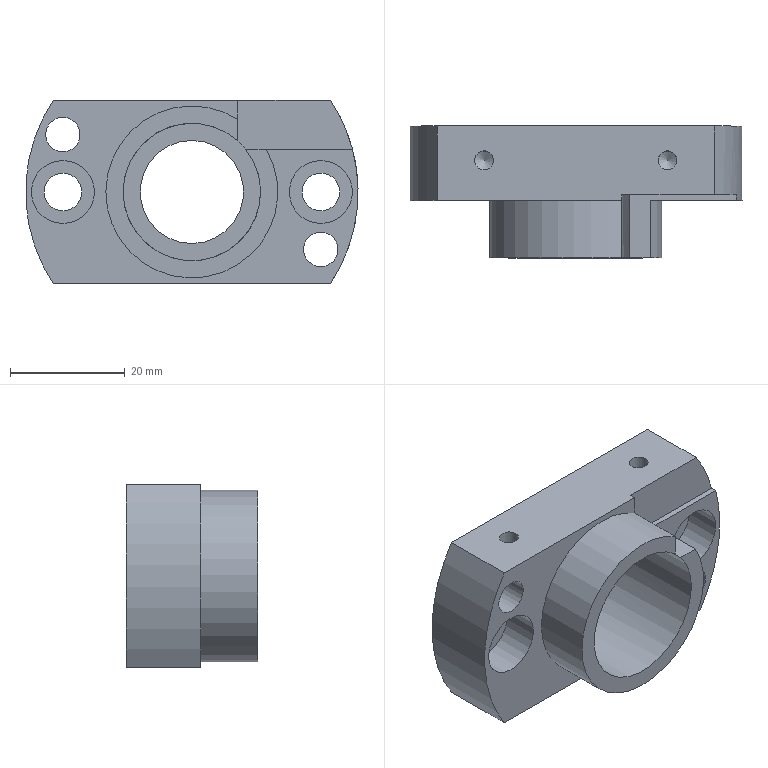Part | NX | features BREP 1 | 1 solid | 26 faces | box 58 x 23 x 32 mm | volume 17221 mm3 | cylinder 13 | plane 11 | cone 2 | commonest cylinder face diameters 3.3 x2 6 x2 6.6 x2 11 x2 58 x2 18 x1
STEP:
#1=CARTESIAN_POINT('',(9.367,11.,7.5));
#2=VERTEX_POINT('',#1);
#3=CARTESIAN_POINT('',(8.,11.,8.944));
#4=VERTEX_POINT('',#3);
#5=CARTESIAN_POINT('',(0.,11.,0.));
#6=DIRECTION('',(0.,-1.,0.));
#7=DIRECTION('',(0.,0.,1.));
#8=AXIS2_PLACEMENT_3D('',#5,#6,#7);
#9=CIRCLE('',#8,12.);
#10=EDGE_CURVE('',#2,#4,#9,.T.);
#11=ORIENTED_EDGE('',*,*,#10,.T.);
#12=CARTESIAN_POINT('',(8.,0.,8.944));
#13=VERTEX_POINT('',#12);
#14=CARTESIAN_POINT('',(8.,0.,8.944));
#15=DIRECTION('',(0.,-1.,0.));
#16=VECTOR('',#15,1000.);
#17=LINE('',#14,#16);
#18=EDGE_CURVE('',#4,#13,#17,.T.);
#19=ORIENTED_EDGE('',*,*,#18,.T.);
#20=CARTESIAN_POINT('',(9.367,0.,7.5));
#21=VERTEX_POINT('',#20);
#22=CARTESIAN_POINT('',(0.,0.,0.));
#23=DIRECTION('',(0.,1.,0.));
#24=DIRECTION('',(0.,0.,1.));
#25=AXIS2_PLACEMENT_3D('',#22,#23,#24);
#26=CIRCLE('',#25,12.);
#27=EDGE_CURVE('',#21,#13,#26,.T.);
#28=ORIENTED_EDGE('',*,*,#27,.F.);
#29=CARTESIAN_POINT('',(9.367,0.,7.5));
#30=DIRECTION('',(0.,1.,0.));
#31=VECTOR('',#30,1000.);
#32=LINE('',#29,#31);
#33=EDGE_CURVE('',#21,#2,#32,.T.);
#34=ORIENTED_EDGE('',*,*,#33,.T.);
#35=EDGE_LOOP('',(#11,#19,#28,#34));
#36=FACE_BOUND('',#35,.T.);
#37=CARTESIAN_POINT('',(0.,20.,12.));
#38=VERTEX_POINT('',#37);
#39=CARTESIAN_POINT('',(0.,20.,0.));
#40=DIRECTION('',(0.,-1.,0.));
#41=DIRECTION('',(0.,0.,1.));
#42=AXIS2_PLACEMENT_3D('',#39,#40,#41);
#43=CIRCLE('',#42,12.);
#44=EDGE_CURVE('',#38,#38,#43,.T.);
#45=ORIENTED_EDGE('',*,*,#44,.F.);
#46=EDGE_LOOP('',(#45));
#47=FACE_BOUND('',#46,.T.);
#48=CARTESIAN_POINT('',(0.,0.,0.));
#49=DIRECTION('',(0.,1.,0.));
#50=DIRECTION('',(0.,0.,-1.));
#51=AXIS2_PLACEMENT_3D('',#48,#49,#50);
#52=CYLINDRICAL_SURFACE('',#51,12.);
#53=ADVANCED_FACE('',(#36,#47),#52,.F.);
#54=CARTESIAN_POINT('',(-22.5,10.,13.));
#55=VERTEX_POINT('',#54);
#56=CARTESIAN_POINT('',(-22.5,10.,10.));
#57=DIRECTION('',(0.,1.,0.));
#58=DIRECTION('',(0.,0.,1.));
#59=AXIS2_PLACEMENT_3D('',#56,#57,#58);
#60=CIRCLE('',#59,3.);
#61=EDGE_CURVE('',#55,#55,#60,.T.);
#62=ORIENTED_EDGE('',*,*,#61,.T.);
#63=EDGE_LOOP('',(#62));
#64=FACE_BOUND('',#63,.T.);
#65=CARTESIAN_POINT('',(22.5,10.,-7.));
#66=VERTEX_POINT('',#65);
#67=CARTESIAN_POINT('',(22.5,10.,-10.));
#68=DIRECTION('',(0.,1.,0.));
#69=DIRECTION('',(0.,0.,1.));
#70=AXIS2_PLACEMENT_3D('',#67,#68,#69);
#71=CIRCLE('',#70,3.);
#72=EDGE_CURVE('',#66,#66,#71,.T.);
#73=ORIENTED_EDGE('',*,*,#72,.T.);
#74=EDGE_LOOP('',(#73));
#75=FACE_BOUND('',#74,.T.);
#76=CARTESIAN_POINT('',(22.5,10.,-5.5));
#77=VERTEX_POINT('',#76);
#78=CARTESIAN_POINT('',(22.5,10.,0.));
#79=DIRECTION('',(0.,-1.,0.));
#80=DIRECTION('',(0.,0.,-1.));
#81=AXIS2_PLACEMENT_3D('',#78,#79,#80);
#82=CIRCLE('',#81,5.5);
#83=EDGE_CURVE('',#77,#77,#82,.T.);
#84=ORIENTED_EDGE('',*,*,#83,.F.);
#85=EDGE_LOOP('',(#84));
#86=FACE_BOUND('',#85,.T.);
#87=CARTESIAN_POINT('',(-22.5,10.,-5.5));
#88=VERTEX_POINT('',#87);
#89=CARTESIAN_POINT('',(-22.5,10.,0.));
#90=DIRECTION('',(0.,-1.,0.));
#91=DIRECTION('',(0.,0.,-1.));
#92=AXIS2_PLACEMENT_3D('',#89,#90,#91);
#93=CIRCLE('',#92,5.5);
#94=EDGE_CURVE('',#88,#88,#93,.T.);
#95=ORIENTED_EDGE('',*,*,#94,.F.);
#96=EDGE_LOOP('',(#95));
#97=FACE_BOUND('',#96,.T.);
#98=CARTESIAN_POINT('',(12.99,10.,7.5));
#99=VERTEX_POINT('',#98);
#100=CARTESIAN_POINT('',(8.,10.,12.689));
#101=VERTEX_POINT('',#100);
#102=CARTESIAN_POINT('',(0.,10.,0.));
#103=DIRECTION('',(0.,1.,0.));
#104=DIRECTION('',(0.,0.,1.));
#105=AXIS2_PLACEMENT_3D('',#102,#103,#104);
#106=CIRCLE('',#105,15.);
#107=EDGE_CURVE('',#99,#101,#106,.T.);
#108=ORIENTED_EDGE('',*,*,#107,.T.);
#109=CARTESIAN_POINT('',(8.,10.,16.));
#110=VERTEX_POINT('',#109);
#111=CARTESIAN_POINT('',(8.,10.,0.));
#112=DIRECTION('',(0.,0.,1.));
#113=VECTOR('',#112,1000.);
#114=LINE('',#111,#113);
#115=EDGE_CURVE('',#101,#110,#114,.T.);
#116=ORIENTED_EDGE('',*,*,#115,.T.);
#117=CARTESIAN_POINT('',(-24.187,10.,16.));
#118=VERTEX_POINT('',#117);
#119=CARTESIAN_POINT('',(-24.187,10.,16.));
#120=DIRECTION('',(1.,0.,0.));
#121=VECTOR('',#120,1000.);
#122=LINE('',#119,#121);
#123=EDGE_CURVE('',#118,#110,#122,.T.);
#124=ORIENTED_EDGE('',*,*,#123,.F.);
#125=CARTESIAN_POINT('',(-24.187,10.,-16.));
#126=VERTEX_POINT('',#125);
#127=CARTESIAN_POINT('',(0.,10.,0.));
#128=DIRECTION('',(0.,1.,0.));
#129=DIRECTION('',(0.,0.,1.));
#130=AXIS2_PLACEMENT_3D('',#127,#128,#129);
#131=CIRCLE('',#130,29.);
#132=EDGE_CURVE('',#126,#118,#131,.T.);
#133=ORIENTED_EDGE('',*,*,#132,.F.);
#134=CARTESIAN_POINT('',(24.187,10.,-16.));
#135=VERTEX_POINT('',#134);
#136=CARTESIAN_POINT('',(-24.187,10.,-16.));
#137=DIRECTION('',(1.,0.,0.));
#138=VECTOR('',#137,1000.);
#139=LINE('',#136,#138);
#140=EDGE_CURVE('',#126,#135,#139,.T.);
#141=ORIENTED_EDGE('',*,*,#140,.T.);
#142=CARTESIAN_POINT('',(28.013,10.,7.5));
#143=VERTEX_POINT('',#142);
#144=CARTESIAN_POINT('',(0.,10.,0.));
#145=DIRECTION('',(0.,1.,0.));
#146=DIRECTION('',(0.,0.,1.));
#147=AXIS2_PLACEMENT_3D('',#144,#145,#146);
#148=CIRCLE('',#147,29.);
#149=EDGE_CURVE('',#143,#135,#148,.T.);
#150=ORIENTED_EDGE('',*,*,#149,.F.);
#151=CARTESIAN_POINT('',(15.,10.,7.5));
#152=DIRECTION('',(-1.,0.,0.));
#153=VECTOR('',#152,1000.);
#154=LINE('',#151,#153);
#155=EDGE_CURVE('',#143,#99,#154,.T.);
#156=ORIENTED_EDGE('',*,*,#155,.T.);
#157=EDGE_LOOP('',(#108,#116,#124,#133,#141,#150,#156));
#158=FACE_BOUND('',#157,.T.);
#159=CARTESIAN_POINT('',(15.,10.,0.));
#160=DIRECTION('',(0.,1.,0.));
#161=DIRECTION('',(0.,0.,-1.));
#162=AXIS2_PLACEMENT_3D('',#159,#160,#161);
#163=PLANE('',#162);
#164=ADVANCED_FACE('',(#64,#75,#86,#97,#158),#163,.F.);
#165=CARTESIAN_POINT('',(24.187,11.,16.));
#166=VERTEX_POINT('',#165);
#167=CARTESIAN_POINT('',(28.013,11.,7.5));
#168=VERTEX_POINT('',#167);
#169=CARTESIAN_POINT('',(0.,11.,0.));
#170=DIRECTION('',(0.,1.,0.));
#171=DIRECTION('',(0.,0.,1.));
#172=AXIS2_PLACEMENT_3D('',#169,#170,#171);
#173=CIRCLE('',#172,29.);
#174=EDGE_CURVE('',#166,#168,#173,.T.);
#175=ORIENTED_EDGE('',*,*,#174,.T.);
#176=CARTESIAN_POINT('',(28.013,0.,7.5));
#177=DIRECTION('',(0.,-1.,0.));
#178=VECTOR('',#177,1000.);
#179=LINE('',#176,#178);
#180=EDGE_CURVE('',#168,#143,#179,.T.);
#181=ORIENTED_EDGE('',*,*,#180,.T.);
#182=ORIENTED_EDGE('',*,*,#149,.T.);
#183=CARTESIAN_POINT('',(24.187,23.,-16.));
#184=VERTEX_POINT('',#183);
#185=CARTESIAN_POINT('',(24.187,73.737,-16.));
#186=DIRECTION('',(0.,-1.,0.));
#187=VECTOR('',#186,1000.);
#188=LINE('',#185,#187);
#189=EDGE_CURVE('',#184,#135,#188,.T.);
#190=ORIENTED_EDGE('',*,*,#189,.F.);
#191=CARTESIAN_POINT('',(24.187,23.,16.));
#192=VERTEX_POINT('',#191);
#193=CARTESIAN_POINT('',(0.,23.,0.));
#194=DIRECTION('',(0.,1.,0.));
#195=DIRECTION('',(0.,0.,1.));
#196=AXIS2_PLACEMENT_3D('',#193,#194,#195);
#197=CIRCLE('',#196,29.);
#198=EDGE_CURVE('',#192,#184,#197,.T.);
#199=ORIENTED_EDGE('',*,*,#198,.F.);
#200=CARTESIAN_POINT('',(24.187,73.737,16.));
#201=DIRECTION('',(0.,-1.,0.));
#202=VECTOR('',#201,1000.);
#203=LINE('',#200,#202);
#204=EDGE_CURVE('',#192,#166,#203,.T.);
#205=ORIENTED_EDGE('',*,*,#204,.T.);
#206=EDGE_LOOP('',(#175,#181,#182,#190,#199,#205));
#207=FACE_BOUND('',#206,.T.);
#208=CARTESIAN_POINT('',(0.,0.,0.));
#209=DIRECTION('',(0.,1.,0.));
#210=DIRECTION('',(0.,0.,-1.));
#211=AXIS2_PLACEMENT_3D('',#208,#209,#210);
#212=CYLINDRICAL_SURFACE('',#211,29.);
#213=ADVANCED_FACE('',(#207),#212,.T.);
#214=CARTESIAN_POINT('',(-24.187,23.,-16.));
#215=VERTEX_POINT('',#214);
#216=CARTESIAN_POINT('',(-24.187,73.737,-16.));
#217=DIRECTION('',(0.,-1.,0.));
#218=VECTOR('',#217,1000.);
#219=LINE('',#216,#218);
#220=EDGE_CURVE('',#215,#126,#219,.T.);
#221=ORIENTED_EDGE('',*,*,#220,.T.);
#222=ORIENTED_EDGE('',*,*,#132,.T.);
#223=CARTESIAN_POINT('',(-24.187,23.,16.));
#224=VERTEX_POINT('',#223);
#225=CARTESIAN_POINT('',(-24.187,73.737,16.));
#226=DIRECTION('',(0.,-1.,0.));
#227=VECTOR('',#226,1000.);
#228=LINE('',#225,#227);
#229=EDGE_CURVE('',#224,#118,#228,.T.);
#230=ORIENTED_EDGE('',*,*,#229,.F.);
#231=CARTESIAN_POINT('',(0.,23.,0.));
#232=DIRECTION('',(0.,1.,0.));
#233=DIRECTION('',(0.,0.,1.));
#234=AXIS2_PLACEMENT_3D('',#231,#232,#233);
#235=CIRCLE('',#234,29.);
#236=EDGE_CURVE('',#215,#224,#235,.T.);
#237=ORIENTED_EDGE('',*,*,#236,.F.);
#238=EDGE_LOOP('',(#221,#222,#230,#237));
#239=FACE_BOUND('',#238,.T.);
#240=CARTESIAN_POINT('',(0.,0.,0.));
#241=DIRECTION('',(0.,1.,0.));
#242=DIRECTION('',(0.,0.,-1.));
#243=AXIS2_PLACEMENT_3D('',#240,#241,#242);
#244=CYLINDRICAL_SURFACE('',#243,29.);
#245=ADVANCED_FACE('',(#239),#244,.T.);
#246=CARTESIAN_POINT('',(-22.5,23.,13.));
#247=VERTEX_POINT('',#246);
#248=CARTESIAN_POINT('',(-22.5,23.,10.));
#249=DIRECTION('',(0.,1.,0.));
#250=DIRECTION('',(0.,0.,1.));
#251=AXIS2_PLACEMENT_3D('',#248,#249,#250);
#252=CIRCLE('',#251,3.);
#253=EDGE_CURVE('',#247,#247,#252,.T.);
#254=ORIENTED_EDGE('',*,*,#253,.F.);
#255=EDGE_LOOP('',(#254));
#256=FACE_BOUND('',#255,.T.);
#257=CARTESIAN_POINT('',(22.5,23.,-7.));
#258=VERTEX_POINT('',#257);
#259=CARTESIAN_POINT('',(22.5,23.,-10.));
#260=DIRECTION('',(0.,1.,0.));
#261=DIRECTION('',(0.,0.,1.));
#262=AXIS2_PLACEMENT_3D('',#259,#260,#261);
#263=CIRCLE('',#262,3.);
#264=EDGE_CURVE('',#258,#258,#263,.T.);
#265=ORIENTED_EDGE('',*,*,#264,.F.);
#266=EDGE_LOOP('',(#265));
#267=FACE_BOUND('',#266,.T.);
#268=CARTESIAN_POINT('',(22.5,23.,-3.3));
#269=VERTEX_POINT('',#268);
#270=CARTESIAN_POINT('',(22.5,23.,0.));
#271=DIRECTION('',(0.,-1.,0.));
#272=DIRECTION('',(0.,0.,-1.));
#273=AXIS2_PLACEMENT_3D('',#270,#271,#272);
#274=CIRCLE('',#273,3.3);
#275=EDGE_CURVE('',#269,#269,#274,.T.);
#276=ORIENTED_EDGE('',*,*,#275,.T.);
#277=EDGE_LOOP('',(#276));
#278=FACE_BOUND('',#277,.T.);
#279=CARTESIAN_POINT('',(-22.5,23.,-3.3));
#280=VERTEX_POINT('',#279);
#281=CARTESIAN_POINT('',(-22.5,23.,0.));
#282=DIRECTION('',(0.,-1.,0.));
#283=DIRECTION('',(0.,0.,-1.));
#284=AXIS2_PLACEMENT_3D('',#281,#282,#283);
#285=CIRCLE('',#284,3.3);
#286=EDGE_CURVE('',#280,#280,#285,.T.);
#287=ORIENTED_EDGE('',*,*,#286,.T.);
#288=EDGE_LOOP('',(#287));
#289=FACE_BOUND('',#288,.T.);
#290=CARTESIAN_POINT('',(-24.187,23.,-16.));
#291=DIRECTION('',(-1.,0.,0.));
#292=VECTOR('',#291,1000.);
#293=LINE('',#290,#292);
#294=EDGE_CURVE('',#184,#215,#293,.T.);
#295=ORIENTED_EDGE('',*,*,#294,.T.);
#296=ORIENTED_EDGE('',*,*,#236,.T.);
#297=CARTESIAN_POINT('',(-24.187,23.,16.));
#298=DIRECTION('',(-1.,0.,0.));
#299=VECTOR('',#298,1000.);
#300=LINE('',#297,#299);
#301=EDGE_CURVE('',#192,#224,#300,.T.);
#302=ORIENTED_EDGE('',*,*,#301,.F.);
#303=ORIENTED_EDGE('',*,*,#198,.T.);
#304=EDGE_LOOP('',(#295,#296,#302,#303));
#305=FACE_BOUND('',#304,.T.);
#306=CARTESIAN_POINT('',(0.,23.,9.));
#307=VERTEX_POINT('',#306);
#308=CARTESIAN_POINT('',(0.,23.,0.));
#309=DIRECTION('',(0.,1.,0.));
#310=DIRECTION('',(0.,0.,1.));
#311=AXIS2_PLACEMENT_3D('',#308,#309,#310);
#312=CIRCLE('',#311,9.);
#313=EDGE_CURVE('',#307,#307,#312,.T.);
#314=ORIENTED_EDGE('',*,*,#313,.F.);
#315=EDGE_LOOP('',(#314));
#316=FACE_BOUND('',#315,.T.);
#317=CARTESIAN_POINT('',(29.,23.,0.));
#318=DIRECTION('',(0.,-1.,0.));
#319=DIRECTION('',(0.,0.,1.));
#320=AXIS2_PLACEMENT_3D('',#317,#318,#319);
#321=PLANE('',#320);
#322=ADVANCED_FACE('',(#256,#267,#278,#289,#305,#316),#321,.F.);
#323=ORIENTED_EDGE('',*,*,#27,.T.);
#324=CARTESIAN_POINT('',(8.,0.,12.689));
#325=VERTEX_POINT('',#324);
#326=CARTESIAN_POINT('',(8.,0.,7.5));
#327=DIRECTION('',(0.,0.,-1.));
#328=VECTOR('',#327,1000.);
#329=LINE('',#326,#328);
#330=EDGE_CURVE('',#325,#13,#329,.T.);
#331=ORIENTED_EDGE('',*,*,#330,.F.);
#332=CARTESIAN_POINT('',(12.99,0.,7.5));
#333=VERTEX_POINT('',#332);
#334=CARTESIAN_POINT('',(0.,0.,0.));
#335=DIRECTION('',(0.,1.,0.));
#336=DIRECTION('',(0.,0.,1.));
#337=AXIS2_PLACEMENT_3D('',#334,#335,#336);
#338=CIRCLE('',#337,15.);
#339=EDGE_CURVE('',#333,#325,#338,.T.);
#340=ORIENTED_EDGE('',*,*,#339,.F.);
#341=CARTESIAN_POINT('',(8.,0.,7.5));
#342=DIRECTION('',(1.,0.,0.));
#343=VECTOR('',#342,1000.);
#344=LINE('',#341,#343);
#345=EDGE_CURVE('',#21,#333,#344,.T.);
#346=ORIENTED_EDGE('',*,*,#345,.F.);
#347=EDGE_LOOP('',(#323,#331,#340,#346));
#348=FACE_BOUND('',#347,.T.);
#349=CARTESIAN_POINT('',(12.,0.,0.));
#350=DIRECTION('',(0.,1.,0.));
#351=DIRECTION('',(0.,0.,-1.));
#352=AXIS2_PLACEMENT_3D('',#349,#350,#351);
#353=PLANE('',#352);
#354=ADVANCED_FACE('',(#348),#353,.F.);
#355=ORIENTED_EDGE('',*,*,#339,.T.);
#356=CARTESIAN_POINT('',(8.,0.,12.689));
#357=DIRECTION('',(0.,1.,0.));
#358=VECTOR('',#357,1000.);
#359=LINE('',#356,#358);
#360=EDGE_CURVE('',#325,#101,#359,.T.);
#361=ORIENTED_EDGE('',*,*,#360,.T.);
#362=ORIENTED_EDGE('',*,*,#107,.F.);
#363=CARTESIAN_POINT('',(12.99,0.,7.5));
#364=DIRECTION('',(0.,-1.,0.));
#365=VECTOR('',#364,1000.);
#366=LINE('',#363,#365);
#367=EDGE_CURVE('',#99,#333,#366,.T.);
#368=ORIENTED_EDGE('',*,*,#367,.T.);
#369=EDGE_LOOP('',(#355,#361,#362,#368));
#370=FACE_BOUND('',#369,.T.);
#371=CARTESIAN_POINT('',(0.,0.,0.));
#372=DIRECTION('',(0.,1.,0.));
#373=DIRECTION('',(0.,0.,-1.));
#374=AXIS2_PLACEMENT_3D('',#371,#372,#373);
#375=CYLINDRICAL_SURFACE('',#374,15.);
#376=ADVANCED_FACE('',(#370),#375,.T.);
#377=CARTESIAN_POINT('',(-14.35,17.,16.));
#378=VERTEX_POINT('',#377);
#379=CARTESIAN_POINT('',(-16.,17.,16.));
#380=DIRECTION('',(0.,0.,1.));
#381=DIRECTION('',(1.,0.,0.));
#382=AXIS2_PLACEMENT_3D('',#379,#380,#381);
#383=CIRCLE('',#382,1.65);
#384=EDGE_CURVE('',#378,#378,#383,.T.);
#385=ORIENTED_EDGE('',*,*,#384,.F.);
#386=EDGE_LOOP('',(#385));
#387=FACE_BOUND('',#386,.T.);
#388=CARTESIAN_POINT('',(17.65,17.,16.));
#389=VERTEX_POINT('',#388);
#390=CARTESIAN_POINT('',(16.,17.,16.));
#391=DIRECTION('',(0.,0.,1.));
#392=DIRECTION('',(1.,0.,0.));
#393=AXIS2_PLACEMENT_3D('',#390,#391,#392);
#394=CIRCLE('',#393,1.65);
#395=EDGE_CURVE('',#389,#389,#394,.T.);
#396=ORIENTED_EDGE('',*,*,#395,.F.);
#397=EDGE_LOOP('',(#396));
#398=FACE_BOUND('',#397,.T.);
#399=ORIENTED_EDGE('',*,*,#123,.T.);
#400=CARTESIAN_POINT('',(8.,11.,16.));
#401=VERTEX_POINT('',#400);
#402=CARTESIAN_POINT('',(8.,11.,16.));
#403=DIRECTION('',(0.,-1.,0.));
#404=VECTOR('',#403,1000.);
#405=LINE('',#402,#404);
#406=EDGE_CURVE('',#401,#110,#405,.T.);
#407=ORIENTED_EDGE('',*,*,#406,.F.);
#408=CARTESIAN_POINT('',(-24.187,11.,16.));
#409=DIRECTION('',(1.,0.,0.));
#410=VECTOR('',#409,1000.);
#411=LINE('',#408,#410);
#412=EDGE_CURVE('',#401,#166,#411,.T.);
#413=ORIENTED_EDGE('',*,*,#412,.T.);
#414=ORIENTED_EDGE('',*,*,#204,.F.);
#415=ORIENTED_EDGE('',*,*,#301,.T.);
#416=ORIENTED_EDGE('',*,*,#229,.T.);
#417=EDGE_LOOP('',(#399,#407,#413,#414,#415,#416));
#418=FACE_BOUND('',#417,.T.);
#419=CARTESIAN_POINT('',(-24.187,73.737,16.));
#420=DIRECTION('',(0.,0.,-1.));
#421=DIRECTION('',(1.,0.,0.));
#422=AXIS2_PLACEMENT_3D('',#419,#420,#421);
#423=PLANE('',#422);
#424=ADVANCED_FACE('',(#387,#398,#418),#423,.F.);
#425=ORIENTED_EDGE('',*,*,#189,.T.);
#426=ORIENTED_EDGE('',*,*,#140,.F.);
#427=ORIENTED_EDGE('',*,*,#220,.F.);
#428=ORIENTED_EDGE('',*,*,#294,.F.);
#429=EDGE_LOOP('',(#425,#426,#427,#428));
#430=FACE_BOUND('',#429,.T.);
#431=CARTESIAN_POINT('',(-24.187,73.737,-16.));
#432=DIRECTION('',(0.,0.,-1.));
#433=DIRECTION('',(1.,0.,0.));
#434=AXIS2_PLACEMENT_3D('',#431,#432,#433);
#435=PLANE('',#434);
#436=ADVANCED_FACE('',(#430),#435,.T.);
#437=ORIENTED_EDGE('',*,*,#286,.F.);
#438=EDGE_LOOP('',(#437));
#439=FACE_BOUND('',#438,.T.);
#440=CARTESIAN_POINT('',(-22.5,16.4,-3.3));
#441=VERTEX_POINT('',#440);
#442=CARTESIAN_POINT('',(-22.5,16.4,0.));
#443=DIRECTION('',(0.,-1.,0.));
#444=DIRECTION('',(0.,0.,-1.));
#445=AXIS2_PLACEMENT_3D('',#442,#443,#444);
#446=CIRCLE('',#445,3.3);
#447=EDGE_CURVE('',#441,#441,#446,.T.);
#448=ORIENTED_EDGE('',*,*,#447,.T.);
#449=EDGE_LOOP('',(#448));
#450=FACE_BOUND('',#449,.T.);
#451=CARTESIAN_POINT('',(-22.5,10.,0.));
#452=DIRECTION('',(0.,-1.,0.));
#453=DIRECTION('',(0.,0.,1.));
#454=AXIS2_PLACEMENT_3D('',#451,#452,#453);
#455=CYLINDRICAL_SURFACE('',#454,3.3);
#456=ADVANCED_FACE('',(#439,#450),#455,.F.);
#457=ORIENTED_EDGE('',*,*,#447,.F.);
#458=EDGE_LOOP('',(#457));
#459=FACE_BOUND('',#458,.T.);
#460=CARTESIAN_POINT('',(-22.5,16.4,-5.5));
#461=VERTEX_POINT('',#460);
#462=CARTESIAN_POINT('',(-22.5,16.4,0.));
#463=DIRECTION('',(0.,-1.,0.));
#464=DIRECTION('',(0.,0.,-1.));
#465=AXIS2_PLACEMENT_3D('',#462,#463,#464);
#466=CIRCLE('',#465,5.5);
#467=EDGE_CURVE('',#461,#461,#466,.T.);
#468=ORIENTED_EDGE('',*,*,#467,.T.);
#469=EDGE_LOOP('',(#468));
#470=FACE_BOUND('',#469,.T.);
#471=CARTESIAN_POINT('',(-19.2,16.4,0.));
#472=DIRECTION('',(0.,1.,0.));
#473=DIRECTION('',(0.,0.,-1.));
#474=AXIS2_PLACEMENT_3D('',#471,#472,#473);
#475=PLANE('',#474);
#476=ADVANCED_FACE('',(#459,#470),#475,.F.);
#477=ORIENTED_EDGE('',*,*,#467,.F.);
#478=EDGE_LOOP('',(#477));
#479=FACE_BOUND('',#478,.T.);
#480=ORIENTED_EDGE('',*,*,#94,.T.);
#481=EDGE_LOOP('',(#480));
#482=FACE_BOUND('',#481,.T.);
#483=CARTESIAN_POINT('',(-22.5,10.,0.));
#484=DIRECTION('',(0.,-1.,0.));
#485=DIRECTION('',(0.,0.,1.));
#486=AXIS2_PLACEMENT_3D('',#483,#484,#485);
#487=CYLINDRICAL_SURFACE('',#486,5.5);
#488=ADVANCED_FACE('',(#479,#482),#487,.F.);
#489=ORIENTED_EDGE('',*,*,#275,.F.);
#490=EDGE_LOOP('',(#489));
#491=FACE_BOUND('',#490,.T.);
#492=CARTESIAN_POINT('',(22.5,16.4,-3.3));
#493=VERTEX_POINT('',#492);
#494=CARTESIAN_POINT('',(22.5,16.4,0.));
#495=DIRECTION('',(0.,-1.,0.));
#496=DIRECTION('',(0.,0.,-1.));
#497=AXIS2_PLACEMENT_3D('',#494,#495,#496);
#498=CIRCLE('',#497,3.3);
#499=EDGE_CURVE('',#493,#493,#498,.T.);
#500=ORIENTED_EDGE('',*,*,#499,.T.);
#501=EDGE_LOOP('',(#500));
#502=FACE_BOUND('',#501,.T.);
#503=CARTESIAN_POINT('',(22.5,10.,0.));
#504=DIRECTION('',(0.,-1.,0.));
#505=DIRECTION('',(0.,0.,1.));
#506=AXIS2_PLACEMENT_3D('',#503,#504,#505);
#507=CYLINDRICAL_SURFACE('',#506,3.3);
#508=ADVANCED_FACE('',(#491,#502),#507,.F.);
#509=ORIENTED_EDGE('',*,*,#499,.F.);
#510=EDGE_LOOP('',(#509));
#511=FACE_BOUND('',#510,.T.);
#512=CARTESIAN_POINT('',(22.5,16.4,-5.5));
#513=VERTEX_POINT('',#512);
#514=CARTESIAN_POINT('',(22.5,16.4,0.));
#515=DIRECTION('',(0.,-1.,0.));
#516=DIRECTION('',(0.,0.,-1.));
#517=AXIS2_PLACEMENT_3D('',#514,#515,#516);
#518=CIRCLE('',#517,5.5);
#519=EDGE_CURVE('',#513,#513,#518,.T.);
#520=ORIENTED_EDGE('',*,*,#519,.T.);
#521=EDGE_LOOP('',(#520));
#522=FACE_BOUND('',#521,.T.);
#523=CARTESIAN_POINT('',(25.8,16.4,0.));
#524=DIRECTION('',(0.,1.,0.));
#525=DIRECTION('',(0.,0.,-1.));
#526=AXIS2_PLACEMENT_3D('',#523,#524,#525);
#527=PLANE('',#526);
#528=ADVANCED_FACE('',(#511,#522),#527,.F.);
#529=ORIENTED_EDGE('',*,*,#519,.F.);
#530=EDGE_LOOP('',(#529));
#531=FACE_BOUND('',#530,.T.);
#532=ORIENTED_EDGE('',*,*,#83,.T.);
#533=EDGE_LOOP('',(#532));
#534=FACE_BOUND('',#533,.T.);
#535=CARTESIAN_POINT('',(22.5,10.,0.));
#536=DIRECTION('',(0.,-1.,0.));
#537=DIRECTION('',(0.,0.,1.));
#538=AXIS2_PLACEMENT_3D('',#535,#536,#537);
#539=CYLINDRICAL_SURFACE('',#538,5.5);
#540=ADVANCED_FACE('',(#531,#534),#539,.F.);
#541=ORIENTED_EDGE('',*,*,#264,.T.);
#542=EDGE_LOOP('',(#541));
#543=FACE_BOUND('',#542,.T.);
#544=ORIENTED_EDGE('',*,*,#72,.F.);
#545=EDGE_LOOP('',(#544));
#546=FACE_BOUND('',#545,.T.);
#547=CARTESIAN_POINT('',(22.5,23.,-10.));
#548=DIRECTION('',(0.,1.,0.));
#549=DIRECTION('',(0.,0.,-1.));
#550=AXIS2_PLACEMENT_3D('',#547,#548,#549);
#551=CYLINDRICAL_SURFACE('',#550,3.);
#552=ADVANCED_FACE('',(#543,#546),#551,.F.);
#553=ORIENTED_EDGE('',*,*,#253,.T.);
#554=EDGE_LOOP('',(#553));
#555=FACE_BOUND('',#554,.T.);
#556=ORIENTED_EDGE('',*,*,#61,.F.);
#557=EDGE_LOOP('',(#556));
#558=FACE_BOUND('',#557,.T.);
#559=CARTESIAN_POINT('',(-22.5,23.,10.));
#560=DIRECTION('',(0.,1.,0.));
#561=DIRECTION('',(0.,0.,-1.));
#562=AXIS2_PLACEMENT_3D('',#559,#560,#561);
#563=CYLINDRICAL_SURFACE('',#562,3.);
#564=ADVANCED_FACE('',(#555,#558),#563,.F.);
#565=CARTESIAN_POINT('',(0.,20.,9.));
#566=VERTEX_POINT('',#565);
#567=CARTESIAN_POINT('',(0.,20.,0.));
#568=DIRECTION('',(0.,1.,0.));
#569=DIRECTION('',(0.,0.,1.));
#570=AXIS2_PLACEMENT_3D('',#567,#568,#569);
#571=CIRCLE('',#570,9.);
#572=EDGE_CURVE('',#566,#566,#571,.T.);
#573=ORIENTED_EDGE('',*,*,#572,.T.);
#574=EDGE_LOOP('',(#573));
#575=FACE_BOUND('',#574,.T.);
#576=ORIENTED_EDGE('',*,*,#44,.T.);
#577=EDGE_LOOP('',(#576));
#578=FACE_BOUND('',#577,.T.);
#579=CARTESIAN_POINT('',(0.,20.,0.));
#580=DIRECTION('',(0.,1.,0.));
#581=DIRECTION('',(0.,0.,-1.));
#582=AXIS2_PLACEMENT_3D('',#579,#580,#581);
#583=PLANE('',#582);
#584=ADVANCED_FACE('',(#575,#578),#583,.F.);
#585=ORIENTED_EDGE('',*,*,#572,.F.);
#586=EDGE_LOOP('',(#585));
#587=FACE_BOUND('',#586,.T.);
#588=ORIENTED_EDGE('',*,*,#313,.T.);
#589=EDGE_LOOP('',(#588));
#590=FACE_BOUND('',#589,.T.);
#591=CARTESIAN_POINT('',(0.,20.,0.));
#592=DIRECTION('',(0.,1.,0.));
#593=DIRECTION('',(0.,0.,-1.));
#594=AXIS2_PLACEMENT_3D('',#591,#592,#593);
#595=CYLINDRICAL_SURFACE('',#594,9.);
#596=ADVANCED_FACE('',(#587,#590),#595,.F.);
#597=ORIENTED_EDGE('',*,*,#345,.T.);
#598=ORIENTED_EDGE('',*,*,#367,.F.);
#599=ORIENTED_EDGE('',*,*,#155,.F.);
#600=ORIENTED_EDGE('',*,*,#180,.F.);
#601=CARTESIAN_POINT('',(8.,11.,7.5));
#602=DIRECTION('',(1.,0.,0.));
#603=VECTOR('',#602,1000.);
#604=LINE('',#601,#603);
#605=EDGE_CURVE('',#2,#168,#604,.T.);
#606=ORIENTED_EDGE('',*,*,#605,.F.);
#607=ORIENTED_EDGE('',*,*,#33,.F.);
#608=EDGE_LOOP('',(#597,#598,#599,#600,#606,#607));
#609=FACE_BOUND('',#608,.T.);
#610=CARTESIAN_POINT('',(8.,11.,7.5));
#611=DIRECTION('',(0.,0.,-1.));
#612=DIRECTION('',(1.,0.,0.));
#613=AXIS2_PLACEMENT_3D('',#610,#611,#612);
#614=PLANE('',#613);
#615=ADVANCED_FACE('',(#609),#614,.F.);
#616=CARTESIAN_POINT('',(8.,11.,7.5));
#617=DIRECTION('',(0.,0.,-1.));
#618=VECTOR('',#617,1000.);
#619=LINE('',#616,#618);
#620=EDGE_CURVE('',#401,#4,#619,.T.);
#621=ORIENTED_EDGE('',*,*,#620,.F.);
#622=ORIENTED_EDGE('',*,*,#406,.T.);
#623=ORIENTED_EDGE('',*,*,#115,.F.);
#624=ORIENTED_EDGE('',*,*,#360,.F.);
#625=ORIENTED_EDGE('',*,*,#330,.T.);
#626=ORIENTED_EDGE('',*,*,#18,.F.);
#627=EDGE_LOOP('',(#621,#622,#623,#624,#625,#626));
#628=FACE_BOUND('',#627,.T.);
#629=CARTESIAN_POINT('',(8.,11.,7.5));
#630=DIRECTION('',(-1.,0.,0.));
#631=DIRECTION('',(0.,0.,-1.));
#632=AXIS2_PLACEMENT_3D('',#629,#630,#631);
#633=PLANE('',#632);
#634=ADVANCED_FACE('',(#628),#633,.F.);
#635=ORIENTED_EDGE('',*,*,#605,.T.);
#636=ORIENTED_EDGE('',*,*,#174,.F.);
#637=ORIENTED_EDGE('',*,*,#412,.F.);
#638=ORIENTED_EDGE('',*,*,#620,.T.);
#639=ORIENTED_EDGE('',*,*,#10,.F.);
#640=EDGE_LOOP('',(#635,#636,#637,#638,#639));
#641=FACE_BOUND('',#640,.T.);
#642=CARTESIAN_POINT('',(0.,11.,0.));
#643=DIRECTION('',(0.,1.,0.));
#644=DIRECTION('',(0.,0.,-1.));
#645=AXIS2_PLACEMENT_3D('',#642,#643,#644);
#646=PLANE('',#645);
#647=ADVANCED_FACE('',(#641),#646,.F.);
#648=CARTESIAN_POINT('',(16.,17.,4.909));
#649=VERTEX_POINT('',#648);
#650=VERTEX_LOOP('',#649);
#651=FACE_BOUND('',#650,.T.);
#652=CARTESIAN_POINT('',(17.65,17.,5.9));
#653=VERTEX_POINT('',#652);
#654=CARTESIAN_POINT('',(16.,17.,5.9));
#655=DIRECTION('',(0.,0.,1.));
#656=DIRECTION('',(1.,0.,0.));
#657=AXIS2_PLACEMENT_3D('',#654,#655,#656);
#658=CIRCLE('',#657,1.65);
#659=EDGE_CURVE('',#653,#653,#658,.T.);
#660=ORIENTED_EDGE('',*,*,#659,.T.);
#661=EDGE_LOOP('',(#660));
#662=FACE_BOUND('',#661,.T.);
#663=CARTESIAN_POINT('',(16.,17.,5.9));
#664=DIRECTION('',(0.,0.,1.));
#665=DIRECTION('',(-1.,0.,0.));
#666=AXIS2_PLACEMENT_3D('',#663,#664,#665);
#667=CONICAL_SURFACE('',#666,1.65,1.03);
#668=ADVANCED_FACE('',(#651,#662),#667,.F.);
#669=ORIENTED_EDGE('',*,*,#659,.F.);
#670=EDGE_LOOP('',(#669));
#671=FACE_BOUND('',#670,.T.);
#672=ORIENTED_EDGE('',*,*,#395,.T.);
#673=EDGE_LOOP('',(#672));
#674=FACE_BOUND('',#673,.T.);
#675=CARTESIAN_POINT('',(16.,17.,16.));
#676=DIRECTION('',(0.,0.,1.));
#677=DIRECTION('',(-1.,0.,0.));
#678=AXIS2_PLACEMENT_3D('',#675,#676,#677);
#679=CYLINDRICAL_SURFACE('',#678,1.65);
#680=ADVANCED_FACE('',(#671,#674),#679,.F.);
#681=CARTESIAN_POINT('',(-16.,17.,4.909));
#682=VERTEX_POINT('',#681);
#683=VERTEX_LOOP('',#682);
#684=FACE_BOUND('',#683,.T.);
#685=CARTESIAN_POINT('',(-14.35,17.,5.9));
#686=VERTEX_POINT('',#685);
#687=CARTESIAN_POINT('',(-16.,17.,5.9));
#688=DIRECTION('',(0.,0.,1.));
#689=DIRECTION('',(1.,0.,0.));
#690=AXIS2_PLACEMENT_3D('',#687,#688,#689);
#691=CIRCLE('',#690,1.65);
#692=EDGE_CURVE('',#686,#686,#691,.T.);
#693=ORIENTED_EDGE('',*,*,#692,.T.);
#694=EDGE_LOOP('',(#693));
#695=FACE_BOUND('',#694,.T.);
#696=CARTESIAN_POINT('',(-16.,17.,5.9));
#697=DIRECTION('',(0.,0.,1.));
#698=DIRECTION('',(-1.,0.,0.));
#699=AXIS2_PLACEMENT_3D('',#696,#697,#698);
#700=CONICAL_SURFACE('',#699,1.65,1.03);
#701=ADVANCED_FACE('',(#684,#695),#700,.F.);
#702=ORIENTED_EDGE('',*,*,#692,.F.);
#703=EDGE_LOOP('',(#702));
#704=FACE_BOUND('',#703,.T.);
#705=ORIENTED_EDGE('',*,*,#384,.T.);
#706=EDGE_LOOP('',(#705));
#707=FACE_BOUND('',#706,.T.);
#708=CARTESIAN_POINT('',(-16.,17.,16.));
#709=DIRECTION('',(0.,0.,1.));
#710=DIRECTION('',(-1.,0.,0.));
#711=AXIS2_PLACEMENT_3D('',#708,#709,#710);
#712=CYLINDRICAL_SURFACE('',#711,1.65);
#713=ADVANCED_FACE('',(#704,#707),#712,.F.);
#714=CLOSED_SHELL('',(#53,#164,#213,#245,#322,#354,#376,#424,#436,#456,#476,#488,#508,#528,#540,#552,#564,#584,#596,#615,#634,#647,#668,#680,#701,#713));
#715=MANIFOLD_SOLID_BREP('',#714);
#716=(LENGTH_UNIT()NAMED_UNIT(*)SI_UNIT(.MILLI.,.METRE.));
#717=UNCERTAINTY_MEASURE_WITH_UNIT(LENGTH_MEASURE(0.00001),#716,'','');
#718=(NAMED_UNIT(*)PLANE_ANGLE_UNIT()SI_UNIT($,.RADIAN.));
#719=(NAMED_UNIT(*)SI_UNIT($,.STERADIAN.)SOLID_ANGLE_UNIT());
#720=(GEOMETRIC_REPRESENTATION_CONTEXT(3)GLOBAL_UNCERTAINTY_ASSIGNED_CONTEXT((#717))GLOBAL_UNIT_ASSIGNED_CONTEXT((#716,#718,#719))REPRESENTATION_CONTEXT('',''));
#721=ADVANCED_BREP_SHAPE_REPRESENTATION('',(#715),#720);